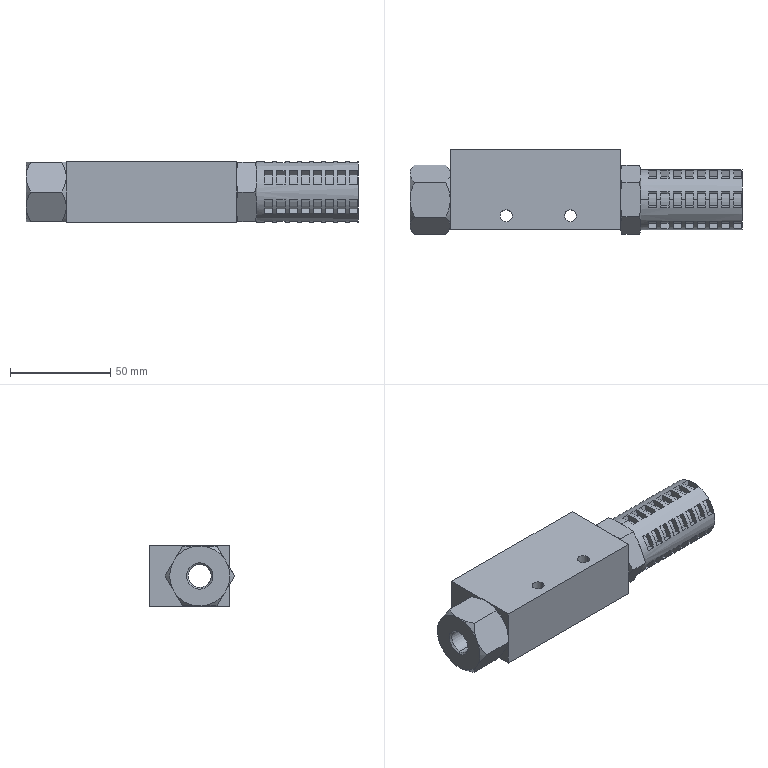Part | STEP file | EV-20 | 1 solid | 312 faces | box 165.5 x 42.263 x 30 mm | volume 136290 mm3 | plane 219 | cylinder 64 | cone 29 | commonest cylinder face diameters 24 x56 6 x4 11.445 x2 30 x2